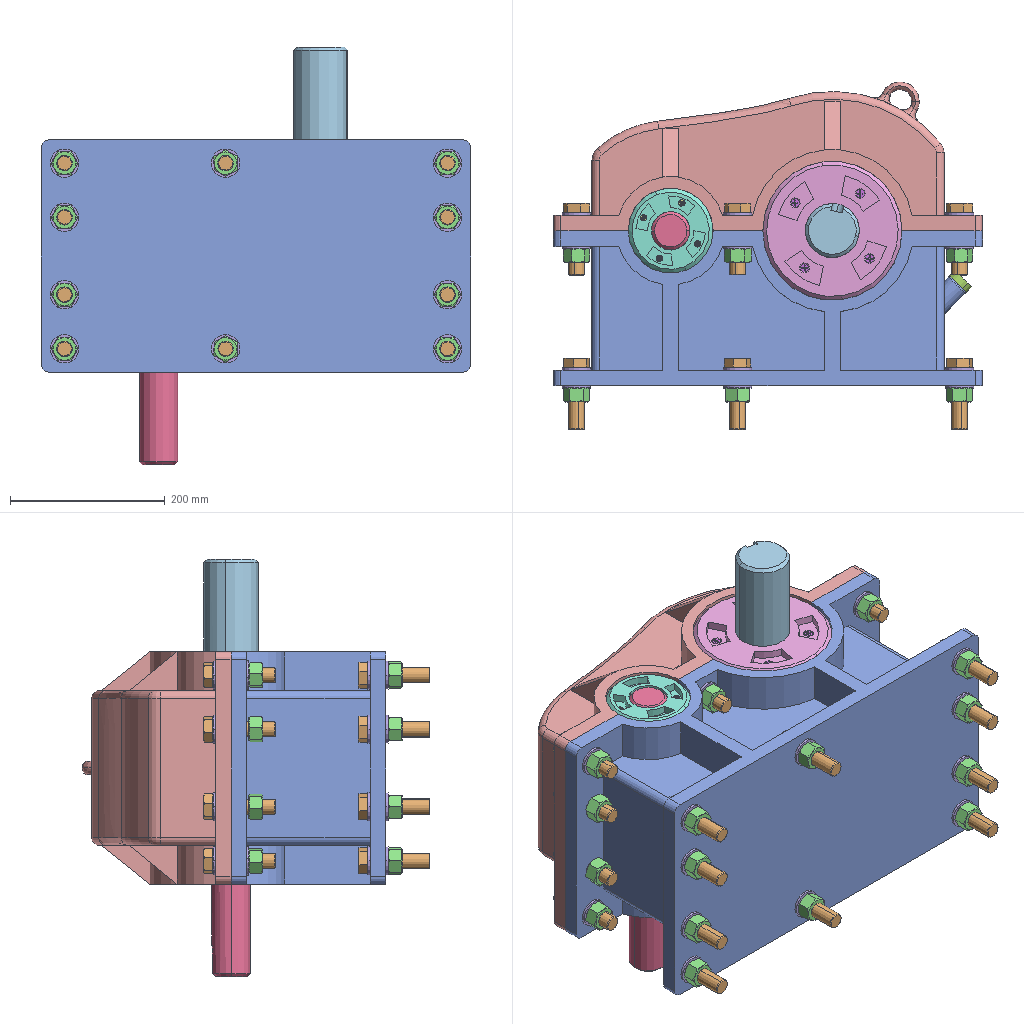Assembly | SolidWorks | 14 different items | 16 placed | box 555 x 449 x 540 mm
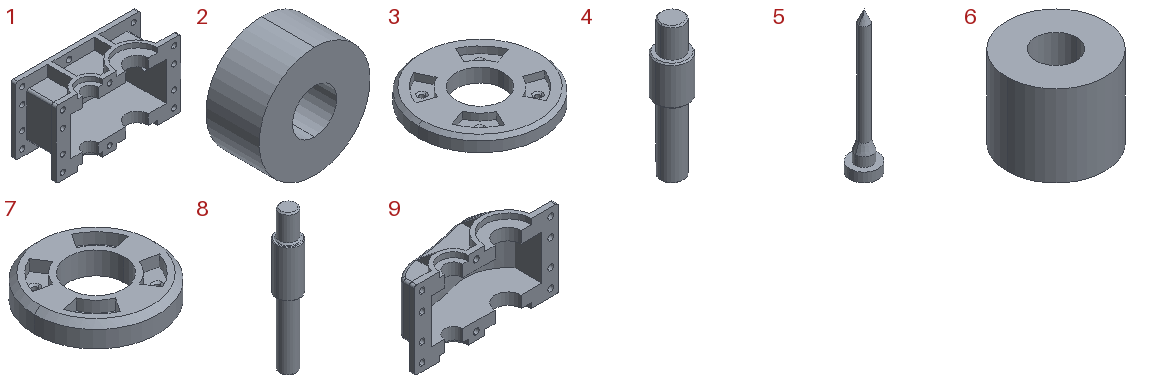Parts list (item | name | quantity | size | volume | features):
1 | - | x1 | 555 x 200 x 300 mm | 8643514 mm3 | features ICE 10, Chamfer 1, Extrusion 1, Fillet 1, MirrorPattern 1, Revolution 1, Shell 1
2 | - | x1 | 250 x 120 x 250 mm | 4948008 mm3 | features Extrusion 1
3 | - | x2 | 180 x 180 x 20 mm | 376159 mm3 | features MirrorPattern 2, Chamfer 1, Extrusion 1, HoleWzd 1, ICE 1
4 | - | x1 | 100 x 100 x 420 mm | 2082883 mm3 | features ICE 2, Chamfer 1, Extrusion 1
5 | - | x1 | 30 x 30 x 150 mm | 22263 mm3 | features Extrusion 1, Revolution 1
6 | - | x1 | 168 x 168 x 140 mm | 2564608 mm3 | features Extrusion 1
7 | - | x2 | 110 x 110 x 20 mm | 126964 mm3 | features MirrorPattern 2, 3DProfileFeature 1, Chamfer 1, Extrusion 1, HoleWzd 1, ICE 1
8 | - | x1 | 70 x 70 x 420 mm | 1082180 mm3 | features Chamfer 3, ICE 2, Extrusion 1
9 | - | x1 | 555 x 192.629 x 300 mm | 5936762 mm3 | features ICE 8, Fillet 4, Extrusion 1, MirrorPattern 1, Shell 1
10 | cross recessed countersunk head screws gb2 | x1 | - | - | -
11 | hex nuts, style 1-grades ab gb | x1 | - | - | -
12 | hexagon head bolts--product grade c gb | x1 | - | - | -
13 | plain washers-n series-grade a gb | x1 | - | - | -
14 | spur gear_gb | x1 | - | - | -
Mates (type | each side: item.copy, entity, surface, feature):
Coincident | 9.1 face plane Boss-Extrude1 | 1.1 face plane Boss-Extrude1
Parallel | 9.1 face plane Boss-Extrude2 | 1.1 face plane Boss-Extrude2
Coincident | 9.1 face plane Boss-Extrude2 | 1.1 face plane Boss-Extrude2 | 2 times
Coincident | 1.1 face plane Revolve1 | 5.1 face plane Boss-Extrude1
Concentric | 9.1 face cylinder Mirror1 | 3.1 face cylinder Boss-Extrude1
Coincident | 9.1 face plane Mirror1 | 3.1 face plane Boss-Extrude1
Concentric | 1.1 face cylinder Cut-Extrude3 | 7.1 face cylinder Boss-Extrude1
Coincident | 1.1 face plane Cut-Extrude1 | 7.1 face plane Boss-Extrude1
Concentric | 3.2 face cylinder Boss-Extrude1 | 4.1 face cylinder Boss-Extrude1
Concentric | 1.1 face cylinder Cut-Extrude3 | 8.1 face cylinder Boss-Extrude1
Coincident | 7.2 face plane Boss-Extrude1 | 8.1 face plane Boss-Extrude1
Coincident | 3.1 face plane Boss-Extrude1 | 4.1 face plane Boss-Extrude1